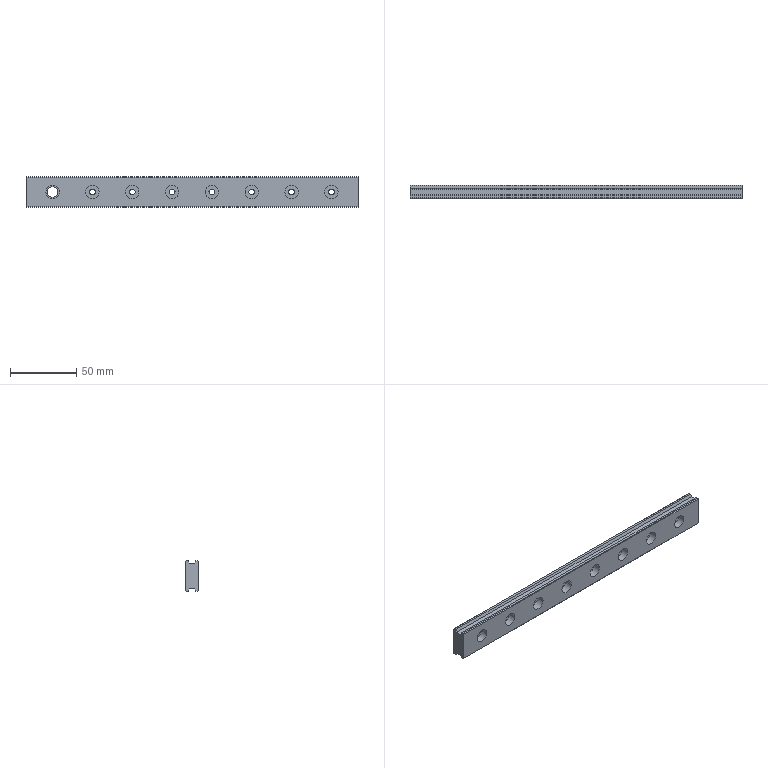Part | STEP file | 1 solid | 42 faces | box 250 x 10 x 23.2 mm | volume 48160 mm3 | plane 26 | cylinder 16 | commonest cylinder face diameters 10 x8 4.5 x7 8 x1